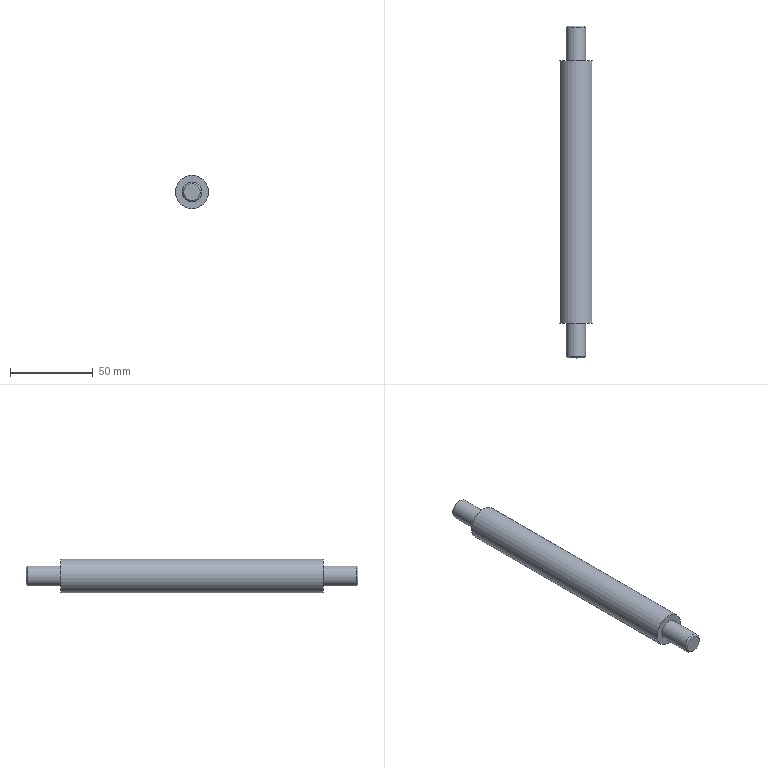Part | STEP file | YBQDJ-DX-4 | 1 solid | 9 faces | box 20 x 200 x 20 mm | volume 54352 mm3 | plane 4 | cylinder 3 | cone 2 | commonest cylinder face diameters 12 x2 20 x1
STEP:
#1=CARTESIAN_POINT('',(0.,0.,0.));
#2=DIRECTION('',(0.,0.,1.));
#3=DIRECTION('',(1.,0.,0.));
#4=AXIS2_PLACEMENT_3D('',#1,#2,#3);
#5=CARTESIAN_POINT('',(441.5,384.,130.));
#6=VERTEX_POINT('',#5);
#7=CARTESIAN_POINT('',(441.5,384.,150.));
#8=VERTEX_POINT('',#7);
#9=CARTESIAN_POINT('',(441.5,384.,140.));
#10=DIRECTION('',(0.,1.,0.));
#11=DIRECTION('',(0.,0.,1.));
#12=AXIS2_PLACEMENT_3D('',#9,#10,#11);
#13=CIRCLE('',#12,10.);
#14=CARTESIAN_POINT('',(441.5,260.,140.));
#15=DIRECTION('',(0.,1.,0.));
#16=DIRECTION('',(0.,0.,-1.));
#17=AXIS2_PLACEMENT_3D('',#14,#15,#16);
#18=CYLINDRICAL_SURFACE('',#17,10.);
#19=CARTESIAN_POINT('',(-3.142,124.));
#20=DIRECTION('',(1.,0.));
#21=VECTOR('',#20,1.);
#22=LINE('',#19,#21);
#23=(GEOMETRIC_REPRESENTATION_CONTEXT(2)PARAMETRIC_REPRESENTATION_CONTEXT()REPRESENTATION_CONTEXT('',''));
#24=DEFINITIONAL_REPRESENTATION('',(#22),#23);
#25=PCURVE('',#18,#24);
#26=CARTESIAN_POINT('',(441.5,384.,140.));
#27=DIRECTION('',(0.,1.,0.));
#28=DIRECTION('',(0.,0.,-1.));
#29=AXIS2_PLACEMENT_3D('',#26,#27,#28);
#30=PLANE('',#29);
#31=CARTESIAN_POINT('',(0.,0.));
#32=DIRECTION('',(-1.,0.));
#33=AXIS2_PLACEMENT_2D('',#31,#32);
#34=CIRCLE('',#33,10.);
#35=(GEOMETRIC_REPRESENTATION_CONTEXT(2)PARAMETRIC_REPRESENTATION_CONTEXT()REPRESENTATION_CONTEXT('',''));
#36=DEFINITIONAL_REPRESENTATION('',(#34),#35);
#37=PCURVE('',#30,#36);
#38=SURFACE_CURVE('',#13,(#25,#37),.PCURVE_S1.);
#39=EDGE_CURVE('',#6,#8,#38,.T.);
#40=ORIENTED_EDGE('',*,*,#39,.F.);
#41=CARTESIAN_POINT('',(441.5,226.,130.));
#42=VERTEX_POINT('',#41);
#43=CARTESIAN_POINT('',(441.5,226.,130.));
#44=CARTESIAN_POINT('',(441.5,384.,130.));
#45=B_SPLINE_CURVE_WITH_KNOTS('',1,(#43,#44),.UNSPECIFIED.,.F.,.F.,(2,2),(-34.,124.),.PIECEWISE_BEZIER_KNOTS.);
#46=CARTESIAN_POINT('',(0.,0.));
#47=DIRECTION('',(0.,1.));
#48=VECTOR('',#47,1.);
#49=LINE('',#46,#48);
#50=(GEOMETRIC_REPRESENTATION_CONTEXT(2)PARAMETRIC_REPRESENTATION_CONTEXT()REPRESENTATION_CONTEXT('',''));
#51=DEFINITIONAL_REPRESENTATION('',(#49),#50);
#52=PCURVE('',#18,#51);
#53=CARTESIAN_POINT('',(6.283,0.));
#54=DIRECTION('',(0.,1.));
#55=VECTOR('',#54,1.);
#56=LINE('',#53,#55);
#57=(GEOMETRIC_REPRESENTATION_CONTEXT(2)PARAMETRIC_REPRESENTATION_CONTEXT()REPRESENTATION_CONTEXT('',''));
#58=DEFINITIONAL_REPRESENTATION('',(#56),#57);
#59=PCURVE('',#18,#58);
#60=SEAM_CURVE('',#45,(#52,#59),.PCURVE_S1.);
#61=EDGE_CURVE('',#42,#6,#60,.T.);
#62=ORIENTED_EDGE('',*,*,#61,.F.);
#63=CARTESIAN_POINT('',(441.5,226.,140.));
#64=DIRECTION('',(0.,-1.,0.));
#65=DIRECTION('',(0.,0.,-1.));
#66=AXIS2_PLACEMENT_3D('',#63,#64,#65);
#67=CIRCLE('',#66,10.);
#68=CARTESIAN_POINT('',(6.283,-34.));
#69=DIRECTION('',(-1.,0.));
#70=VECTOR('',#69,1.);
#71=LINE('',#68,#70);
#72=(GEOMETRIC_REPRESENTATION_CONTEXT(2)PARAMETRIC_REPRESENTATION_CONTEXT()REPRESENTATION_CONTEXT('',''));
#73=DEFINITIONAL_REPRESENTATION('',(#71),#72);
#74=PCURVE('',#18,#73);
#75=CARTESIAN_POINT('',(441.5,226.,140.));
#76=DIRECTION('',(0.,-1.,0.));
#77=DIRECTION('',(0.,0.,-1.));
#78=AXIS2_PLACEMENT_3D('',#75,#76,#77);
#79=PLANE('',#78);
#80=CARTESIAN_POINT('',(0.,0.));
#81=DIRECTION('',(1.,0.));
#82=AXIS2_PLACEMENT_2D('',#80,#81);
#83=CIRCLE('',#82,10.);
#84=(GEOMETRIC_REPRESENTATION_CONTEXT(2)PARAMETRIC_REPRESENTATION_CONTEXT()REPRESENTATION_CONTEXT('',''));
#85=DEFINITIONAL_REPRESENTATION('',(#83),#84);
#86=PCURVE('',#79,#85);
#87=SURFACE_CURVE('',#67,(#74,#86),.PCURVE_S1.);
#88=EDGE_CURVE('',#42,#42,#87,.T.);
#89=ORIENTED_EDGE('',*,*,#88,.F.);
#90=ORIENTED_EDGE('',*,*,#61,.T.);
#91=CARTESIAN_POINT('',(441.5,384.,140.));
#92=DIRECTION('',(0.,1.,0.));
#93=DIRECTION('',(0.,0.,1.));
#94=AXIS2_PLACEMENT_3D('',#91,#92,#93);
#95=CIRCLE('',#94,10.);
#96=CARTESIAN_POINT('',(3.142,124.));
#97=DIRECTION('',(1.,0.));
#98=VECTOR('',#97,1.);
#99=LINE('',#96,#98);
#100=(GEOMETRIC_REPRESENTATION_CONTEXT(2)PARAMETRIC_REPRESENTATION_CONTEXT()REPRESENTATION_CONTEXT('',''));
#101=DEFINITIONAL_REPRESENTATION('',(#99),#100);
#102=PCURVE('',#18,#101);
#103=CARTESIAN_POINT('',(0.,0.));
#104=DIRECTION('',(-1.,0.));
#105=AXIS2_PLACEMENT_2D('',#103,#104);
#106=CIRCLE('',#105,10.);
#107=(GEOMETRIC_REPRESENTATION_CONTEXT(2)PARAMETRIC_REPRESENTATION_CONTEXT()REPRESENTATION_CONTEXT('',''));
#108=DEFINITIONAL_REPRESENTATION('',(#106),#107);
#109=PCURVE('',#30,#108);
#110=SURFACE_CURVE('',#95,(#102,#109),.PCURVE_S1.);
#111=EDGE_CURVE('',#8,#6,#110,.T.);
#112=ORIENTED_EDGE('',*,*,#111,.F.);
#113=EDGE_LOOP('',(#40,#62,#89,#90,#112));
#114=FACE_BOUND('',#113,.T.);
#115=ADVANCED_FACE('',(#114),#18,.T.);
#116=CARTESIAN_POINT('',(441.5,384.,146.));
#117=VERTEX_POINT('',#116);
#118=CARTESIAN_POINT('',(441.5,384.,140.));
#119=DIRECTION('',(0.,-1.,0.));
#120=DIRECTION('',(0.,0.,1.));
#121=AXIS2_PLACEMENT_3D('',#118,#119,#120);
#122=CIRCLE('',#121,6.);
#123=CARTESIAN_POINT('',(-6.,0.));
#124=CARTESIAN_POINT('',(-6.,10.392));
#125=CARTESIAN_POINT('',(3.,5.196));
#126=CARTESIAN_POINT('',(12.,0.));
#127=CARTESIAN_POINT('',(3.,-5.196));
#128=CARTESIAN_POINT('',(-6.,-10.392));
#129=CARTESIAN_POINT('',(-6.,0.));
#130=(BOUNDED_CURVE()B_SPLINE_CURVE(2,(#123,#124,#125,#126,#127,#128,#129),.UNSPECIFIED.,.T.,.F.)B_SPLINE_CURVE_WITH_KNOTS((1,2,2,2,2,1),(-2.094,0.,2.094,4.189,6.283,8.378),.UNSPECIFIED.)CURVE()GEOMETRIC_REPRESENTATION_ITEM()RATIONAL_B_SPLINE_CURVE((1.,0.5,1.,0.5,1.,0.5,1.))REPRESENTATION_ITEM(''));
#131=(GEOMETRIC_REPRESENTATION_CONTEXT(2)PARAMETRIC_REPRESENTATION_CONTEXT()REPRESENTATION_CONTEXT('',''));
#132=DEFINITIONAL_REPRESENTATION('',(#130),#131);
#133=PCURVE('',#30,#132);
#134=CARTESIAN_POINT('',(441.5,410.,140.));
#135=DIRECTION('',(0.,-1.,0.));
#136=DIRECTION('',(0.,0.,1.));
#137=AXIS2_PLACEMENT_3D('',#134,#135,#136);
#138=CYLINDRICAL_SURFACE('',#137,6.);
#139=CARTESIAN_POINT('',(0.,26.));
#140=DIRECTION('',(1.,0.));
#141=VECTOR('',#140,1.);
#142=LINE('',#139,#141);
#143=(GEOMETRIC_REPRESENTATION_CONTEXT(2)PARAMETRIC_REPRESENTATION_CONTEXT()REPRESENTATION_CONTEXT('',''));
#144=DEFINITIONAL_REPRESENTATION('',(#142),#143);
#145=PCURVE('',#138,#144);
#146=SURFACE_CURVE('',#122,(#133,#145),.PCURVE_S1.);
#147=EDGE_CURVE('',#117,#117,#146,.T.);
#148=ORIENTED_EDGE('',*,*,#147,.T.);
#149=EDGE_LOOP('',(#148));
#150=FACE_BOUND('',#149,.T.);
#151=ORIENTED_EDGE('',*,*,#111,.T.);
#152=ORIENTED_EDGE('',*,*,#39,.T.);
#153=EDGE_LOOP('',(#151,#152));
#154=FACE_BOUND('',#153,.T.);
#155=ADVANCED_FACE('',(#150,#154),#30,.T.);
#156=CARTESIAN_POINT('',(441.5,404.,134.));
#157=VERTEX_POINT('',#156);
#158=CARTESIAN_POINT('',(441.5,404.,146.));
#159=VERTEX_POINT('',#158);
#160=CARTESIAN_POINT('',(441.5,404.,140.));
#161=DIRECTION('',(0.,-1.,0.));
#162=DIRECTION('',(0.,0.,-1.));
#163=AXIS2_PLACEMENT_3D('',#160,#161,#162);
#164=CIRCLE('',#163,6.);
#165=CARTESIAN_POINT('',(3.142,6.));
#166=DIRECTION('',(1.,0.));
#167=VECTOR('',#166,1.);
#168=LINE('',#165,#167);
#169=(GEOMETRIC_REPRESENTATION_CONTEXT(2)PARAMETRIC_REPRESENTATION_CONTEXT()REPRESENTATION_CONTEXT('',''));
#170=DEFINITIONAL_REPRESENTATION('',(#168),#169);
#171=PCURVE('',#138,#170);
#172=CARTESIAN_POINT('',(441.5,405.,140.));
#173=DIRECTION('',(0.,-1.,0.));
#174=DIRECTION('',(0.,0.,-1.));
#175=AXIS2_PLACEMENT_3D('',#172,#173,#174);
#176=CONICAL_SURFACE('',#175,5.,0.7854);
#177=CARTESIAN_POINT('',(0.,1.));
#178=DIRECTION('',(1.,0.));
#179=VECTOR('',#178,1.);
#180=LINE('',#177,#179);
#181=(GEOMETRIC_REPRESENTATION_CONTEXT(2)PARAMETRIC_REPRESENTATION_CONTEXT()REPRESENTATION_CONTEXT('',''));
#182=DEFINITIONAL_REPRESENTATION('',(#180),#181);
#183=PCURVE('',#176,#182);
#184=SURFACE_CURVE('',#164,(#171,#183),.PCURVE_S1.);
#185=EDGE_CURVE('',#157,#159,#184,.T.);
#186=ORIENTED_EDGE('',*,*,#185,.T.);
#187=CARTESIAN_POINT('',(441.5,404.,146.));
#188=CARTESIAN_POINT('',(441.5,384.,146.));
#189=B_SPLINE_CURVE_WITH_KNOTS('',1,(#187,#188),.UNSPECIFIED.,.F.,.F.,(2,2),(6.,26.),.PIECEWISE_BEZIER_KNOTS.);
#190=CARTESIAN_POINT('',(6.283,0.));
#191=DIRECTION('',(0.,1.));
#192=VECTOR('',#191,1.);
#193=LINE('',#190,#192);
#194=(GEOMETRIC_REPRESENTATION_CONTEXT(2)PARAMETRIC_REPRESENTATION_CONTEXT()REPRESENTATION_CONTEXT('',''));
#195=DEFINITIONAL_REPRESENTATION('',(#193),#194);
#196=PCURVE('',#138,#195);
#197=CARTESIAN_POINT('',(0.,0.));
#198=DIRECTION('',(0.,1.));
#199=VECTOR('',#198,1.);
#200=LINE('',#197,#199);
#201=(GEOMETRIC_REPRESENTATION_CONTEXT(2)PARAMETRIC_REPRESENTATION_CONTEXT()REPRESENTATION_CONTEXT('',''));
#202=DEFINITIONAL_REPRESENTATION('',(#200),#201);
#203=PCURVE('',#138,#202);
#204=SEAM_CURVE('',#189,(#196,#203),.PCURVE_S1.);
#205=EDGE_CURVE('',#159,#117,#204,.T.);
#206=ORIENTED_EDGE('',*,*,#205,.T.);
#207=ORIENTED_EDGE('',*,*,#147,.F.);
#208=ORIENTED_EDGE('',*,*,#205,.F.);
#209=CARTESIAN_POINT('',(441.5,404.,140.));
#210=DIRECTION('',(0.,-1.,0.));
#211=DIRECTION('',(0.,0.,-1.));
#212=AXIS2_PLACEMENT_3D('',#209,#210,#211);
#213=CIRCLE('',#212,6.);
#214=CARTESIAN_POINT('',(-3.142,6.));
#215=DIRECTION('',(1.,0.));
#216=VECTOR('',#215,1.);
#217=LINE('',#214,#216);
#218=(GEOMETRIC_REPRESENTATION_CONTEXT(2)PARAMETRIC_REPRESENTATION_CONTEXT()REPRESENTATION_CONTEXT('',''));
#219=DEFINITIONAL_REPRESENTATION('',(#217),#218);
#220=PCURVE('',#138,#219);
#221=CARTESIAN_POINT('',(0.,1.));
#222=DIRECTION('',(1.,0.));
#223=VECTOR('',#222,1.);
#224=LINE('',#221,#223);
#225=(GEOMETRIC_REPRESENTATION_CONTEXT(2)PARAMETRIC_REPRESENTATION_CONTEXT()REPRESENTATION_CONTEXT('',''));
#226=DEFINITIONAL_REPRESENTATION('',(#224),#225);
#227=PCURVE('',#176,#226);
#228=SURFACE_CURVE('',#213,(#220,#227),.PCURVE_S1.);
#229=EDGE_CURVE('',#159,#157,#228,.T.);
#230=ORIENTED_EDGE('',*,*,#229,.T.);
#231=EDGE_LOOP('',(#186,#206,#207,#208,#230));
#232=FACE_BOUND('',#231,.T.);
#233=ADVANCED_FACE('',(#232),#138,.T.);
#234=CARTESIAN_POINT('',(446.5,405.,140.));
#235=VERTEX_POINT('',#234);
#236=CARTESIAN_POINT('',(441.5,405.,135.));
#237=VERTEX_POINT('',#236);
#238=CARTESIAN_POINT('',(441.5,405.,140.));
#239=DIRECTION('',(0.,1.,0.));
#240=DIRECTION('',(1.,0.,0.));
#241=AXIS2_PLACEMENT_3D('',#238,#239,#240);
#242=CIRCLE('',#241,5.);
#243=CARTESIAN_POINT('',(466.5,405.,20.));
#244=DIRECTION('',(0.,-1.,0.));
#245=DIRECTION('',(0.,0.,1.));
#246=AXIS2_PLACEMENT_3D('',#243,#244,#245);
#247=PLANE('',#246);
#248=CARTESIAN_POINT('',(120.,20.));
#249=CARTESIAN_POINT('',(111.34,20.));
#250=CARTESIAN_POINT('',(115.67,27.5));
#251=CARTESIAN_POINT('',(120.,35.));
#252=CARTESIAN_POINT('',(124.33,27.5));
#253=CARTESIAN_POINT('',(128.66,20.));
#254=CARTESIAN_POINT('',(120.,20.));
#255=(BOUNDED_CURVE()B_SPLINE_CURVE(2,(#248,#249,#250,#251,#252,#253,#254),.UNSPECIFIED.,.T.,.F.)B_SPLINE_CURVE_WITH_KNOTS((1,2,2,2,2,1),(-2.094,0.,2.094,4.189,6.283,8.378),.UNSPECIFIED.)CURVE()GEOMETRIC_REPRESENTATION_ITEM()RATIONAL_B_SPLINE_CURVE((1.,0.5,1.,0.5,1.,0.5,1.))REPRESENTATION_ITEM(''));
#256=(GEOMETRIC_REPRESENTATION_CONTEXT(2)PARAMETRIC_REPRESENTATION_CONTEXT()REPRESENTATION_CONTEXT('',''));
#257=DEFINITIONAL_REPRESENTATION('',(#255),#256);
#258=PCURVE('',#247,#257);
#259=CARTESIAN_POINT('',(1.571,0.));
#260=DIRECTION('',(-1.,0.));
#261=VECTOR('',#260,1.);
#262=LINE('',#259,#261);
#263=(GEOMETRIC_REPRESENTATION_CONTEXT(2)PARAMETRIC_REPRESENTATION_CONTEXT()REPRESENTATION_CONTEXT('',''));
#264=DEFINITIONAL_REPRESENTATION('',(#262),#263);
#265=PCURVE('',#176,#264);
#266=SURFACE_CURVE('',#242,(#258,#265),.PCURVE_S1.);
#267=EDGE_CURVE('',#235,#237,#266,.T.);
#268=ORIENTED_EDGE('',*,*,#267,.T.);
#269=CARTESIAN_POINT('',(441.5,405.,140.));
#270=DIRECTION('',(0.,1.,0.));
#271=DIRECTION('',(1.,0.,0.));
#272=AXIS2_PLACEMENT_3D('',#269,#270,#271);
#273=CIRCLE('',#272,5.);
#274=CARTESIAN_POINT('',(120.,20.));
#275=CARTESIAN_POINT('',(111.34,20.));
#276=CARTESIAN_POINT('',(115.67,27.5));
#277=CARTESIAN_POINT('',(120.,35.));
#278=CARTESIAN_POINT('',(124.33,27.5));
#279=CARTESIAN_POINT('',(128.66,20.));
#280=CARTESIAN_POINT('',(120.,20.));
#281=(BOUNDED_CURVE()B_SPLINE_CURVE(2,(#274,#275,#276,#277,#278,#279,#280),.UNSPECIFIED.,.T.,.F.)B_SPLINE_CURVE_WITH_KNOTS((1,2,2,2,2,1),(-2.094,0.,2.094,4.189,6.283,8.378),.UNSPECIFIED.)CURVE()GEOMETRIC_REPRESENTATION_ITEM()RATIONAL_B_SPLINE_CURVE((1.,0.5,1.,0.5,1.,0.5,1.))REPRESENTATION_ITEM(''));
#282=(GEOMETRIC_REPRESENTATION_CONTEXT(2)PARAMETRIC_REPRESENTATION_CONTEXT()REPRESENTATION_CONTEXT('',''));
#283=DEFINITIONAL_REPRESENTATION('',(#281),#282);
#284=PCURVE('',#247,#283);
#285=CARTESIAN_POINT('',(7.854,0.));
#286=DIRECTION('',(-1.,0.));
#287=VECTOR('',#286,1.);
#288=LINE('',#285,#287);
#289=(GEOMETRIC_REPRESENTATION_CONTEXT(2)PARAMETRIC_REPRESENTATION_CONTEXT()REPRESENTATION_CONTEXT('',''));
#290=DEFINITIONAL_REPRESENTATION('',(#288),#289);
#291=PCURVE('',#176,#290);
#292=SURFACE_CURVE('',#273,(#284,#291),.PCURVE_S1.);
#293=EDGE_CURVE('',#237,#235,#292,.T.);
#294=ORIENTED_EDGE('',*,*,#293,.T.);
#295=EDGE_LOOP('',(#268,#294));
#296=FACE_BOUND('',#295,.T.);
#297=ADVANCED_FACE('',(#296),#247,.F.);
#298=CARTESIAN_POINT('',(441.5,226.,134.));
#299=VERTEX_POINT('',#298);
#300=CARTESIAN_POINT('',(441.5,226.,146.));
#301=VERTEX_POINT('',#300);
#302=CARTESIAN_POINT('',(441.5,226.,140.));
#303=DIRECTION('',(0.,1.,0.));
#304=DIRECTION('',(0.,0.,-1.));
#305=AXIS2_PLACEMENT_3D('',#302,#303,#304);
#306=CIRCLE('',#305,6.);
#307=CARTESIAN_POINT('',(6.,0.));
#308=CARTESIAN_POINT('',(6.,-10.392));
#309=CARTESIAN_POINT('',(-3.,-5.196));
#310=CARTESIAN_POINT('',(-12.,0.));
#311=CARTESIAN_POINT('',(-3.,5.196));
#312=CARTESIAN_POINT('',(6.,10.392));
#313=CARTESIAN_POINT('',(6.,0.));
#314=(BOUNDED_CURVE()B_SPLINE_CURVE(2,(#307,#308,#309,#310,#311,#312,#313),.UNSPECIFIED.,.T.,.F.)B_SPLINE_CURVE_WITH_KNOTS((1,2,2,2,2,1),(-2.094,0.,2.094,4.189,6.283,8.378),.UNSPECIFIED.)CURVE()GEOMETRIC_REPRESENTATION_ITEM()RATIONAL_B_SPLINE_CURVE((1.,0.5,1.,0.5,1.,0.5,1.))REPRESENTATION_ITEM(''));
#315=(GEOMETRIC_REPRESENTATION_CONTEXT(2)PARAMETRIC_REPRESENTATION_CONTEXT()REPRESENTATION_CONTEXT('',''));
#316=DEFINITIONAL_REPRESENTATION('',(#314),#315);
#317=PCURVE('',#79,#316);
#318=CARTESIAN_POINT('',(441.5,200.,140.));
#319=DIRECTION('',(0.,1.,0.));
#320=DIRECTION('',(0.,0.,1.));
#321=AXIS2_PLACEMENT_3D('',#318,#319,#320);
#322=CYLINDRICAL_SURFACE('',#321,6.);
#323=CARTESIAN_POINT('',(3.142,26.));
#324=DIRECTION('',(1.,0.));
#325=VECTOR('',#324,1.);
#326=LINE('',#323,#325);
#327=(GEOMETRIC_REPRESENTATION_CONTEXT(2)PARAMETRIC_REPRESENTATION_CONTEXT()REPRESENTATION_CONTEXT('',''));
#328=DEFINITIONAL_REPRESENTATION('',(#326),#327);
#329=PCURVE('',#322,#328);
#330=SURFACE_CURVE('',#306,(#317,#329),.PCURVE_S1.);
#331=EDGE_CURVE('',#299,#301,#330,.T.);
#332=ORIENTED_EDGE('',*,*,#331,.T.);
#333=CARTESIAN_POINT('',(441.5,226.,140.));
#334=DIRECTION('',(0.,1.,0.));
#335=DIRECTION('',(0.,0.,-1.));
#336=AXIS2_PLACEMENT_3D('',#333,#334,#335);
#337=CIRCLE('',#336,6.);
#338=CARTESIAN_POINT('',(6.,0.));
#339=CARTESIAN_POINT('',(6.,-10.392));
#340=CARTESIAN_POINT('',(-3.,-5.196));
#341=CARTESIAN_POINT('',(-12.,0.));
#342=CARTESIAN_POINT('',(-3.,5.196));
#343=CARTESIAN_POINT('',(6.,10.392));
#344=CARTESIAN_POINT('',(6.,0.));
#345=(BOUNDED_CURVE()B_SPLINE_CURVE(2,(#338,#339,#340,#341,#342,#343,#344),.UNSPECIFIED.,.T.,.F.)B_SPLINE_CURVE_WITH_KNOTS((1,2,2,2,2,1),(-2.094,0.,2.094,4.189,6.283,8.378),.UNSPECIFIED.)CURVE()GEOMETRIC_REPRESENTATION_ITEM()RATIONAL_B_SPLINE_CURVE((1.,0.5,1.,0.5,1.,0.5,1.))REPRESENTATION_ITEM(''));
#346=(GEOMETRIC_REPRESENTATION_CONTEXT(2)PARAMETRIC_REPRESENTATION_CONTEXT()REPRESENTATION_CONTEXT('',''));
#347=DEFINITIONAL_REPRESENTATION('',(#345),#346);
#348=PCURVE('',#79,#347);
#349=CARTESIAN_POINT('',(-3.142,26.));
#350=DIRECTION('',(1.,0.));
#351=VECTOR('',#350,1.);
#352=LINE('',#349,#351);
#353=(GEOMETRIC_REPRESENTATION_CONTEXT(2)PARAMETRIC_REPRESENTATION_CONTEXT()REPRESENTATION_CONTEXT('',''));
#354=DEFINITIONAL_REPRESENTATION('',(#352),#353);
#355=PCURVE('',#322,#354);
#356=SURFACE_CURVE('',#337,(#348,#355),.PCURVE_S1.);
#357=EDGE_CURVE('',#301,#299,#356,.T.);
#358=ORIENTED_EDGE('',*,*,#357,.T.);
#359=EDGE_LOOP('',(#332,#358));
#360=FACE_BOUND('',#359,.T.);
#361=ORIENTED_EDGE('',*,*,#88,.T.);
#362=EDGE_LOOP('',(#361));
#363=FACE_BOUND('',#362,.T.);
#364=ADVANCED_FACE('',(#360,#363),#79,.T.);
#365=CARTESIAN_POINT('',(441.5,206.,146.));
#366=VERTEX_POINT('',#365);
#367=CARTESIAN_POINT('',(441.5,206.,140.));
#368=DIRECTION('',(0.,1.,0.));
#369=DIRECTION('',(0.,0.,1.));
#370=AXIS2_PLACEMENT_3D('',#367,#368,#369);
#371=CIRCLE('',#370,6.);
#372=CARTESIAN_POINT('',(0.,6.));
#373=DIRECTION('',(1.,0.));
#374=VECTOR('',#373,1.);
#375=LINE('',#372,#374);
#376=(GEOMETRIC_REPRESENTATION_CONTEXT(2)PARAMETRIC_REPRESENTATION_CONTEXT()REPRESENTATION_CONTEXT('',''));
#377=DEFINITIONAL_REPRESENTATION('',(#375),#376);
#378=PCURVE('',#322,#377);
#379=CARTESIAN_POINT('',(441.5,205.,140.));
#380=DIRECTION('',(0.,1.,0.));
#381=DIRECTION('',(0.,0.,1.));
#382=AXIS2_PLACEMENT_3D('',#379,#380,#381);
#383=CONICAL_SURFACE('',#382,5.,0.7854);
#384=CARTESIAN_POINT('',(0.,1.));
#385=DIRECTION('',(1.,0.));
#386=VECTOR('',#385,1.);
#387=LINE('',#384,#386);
#388=(GEOMETRIC_REPRESENTATION_CONTEXT(2)PARAMETRIC_REPRESENTATION_CONTEXT()REPRESENTATION_CONTEXT('',''));
#389=DEFINITIONAL_REPRESENTATION('',(#387),#388);
#390=PCURVE('',#383,#389);
#391=SURFACE_CURVE('',#371,(#378,#390),.PCURVE_S1.);
#392=EDGE_CURVE('',#366,#366,#391,.T.);
#393=ORIENTED_EDGE('',*,*,#392,.T.);
#394=CARTESIAN_POINT('',(441.5,206.,146.));
#395=CARTESIAN_POINT('',(441.5,226.,146.));
#396=B_SPLINE_CURVE_WITH_KNOTS('',1,(#394,#395),.UNSPECIFIED.,.F.,.F.,(2,2),(6.,26.),.PIECEWISE_BEZIER_KNOTS.);
#397=CARTESIAN_POINT('',(6.283,0.));
#398=DIRECTION('',(0.,1.));
#399=VECTOR('',#398,1.);
#400=LINE('',#397,#399);
#401=(GEOMETRIC_REPRESENTATION_CONTEXT(2)PARAMETRIC_REPRESENTATION_CONTEXT()REPRESENTATION_CONTEXT('',''));
#402=DEFINITIONAL_REPRESENTATION('',(#400),#401);
#403=PCURVE('',#322,#402);
#404=CARTESIAN_POINT('',(0.,0.));
#405=DIRECTION('',(0.,1.));
#406=VECTOR('',#405,1.);
#407=LINE('',#404,#406);
#408=(GEOMETRIC_REPRESENTATION_CONTEXT(2)PARAMETRIC_REPRESENTATION_CONTEXT()REPRESENTATION_CONTEXT('',''));
#409=DEFINITIONAL_REPRESENTATION('',(#407),#408);
#410=PCURVE('',#322,#409);
#411=SEAM_CURVE('',#396,(#403,#410),.PCURVE_S1.);
#412=EDGE_CURVE('',#366,#301,#411,.T.);
#413=ORIENTED_EDGE('',*,*,#412,.T.);
#414=ORIENTED_EDGE('',*,*,#331,.F.);
#415=ORIENTED_EDGE('',*,*,#357,.F.);
#416=ORIENTED_EDGE('',*,*,#412,.F.);
#417=EDGE_LOOP('',(#393,#413,#414,#415,#416));
#418=FACE_BOUND('',#417,.T.);
#419=ADVANCED_FACE('',(#418),#322,.T.);
#420=CARTESIAN_POINT('',(441.5,205.,145.));
#421=VERTEX_POINT('',#420);
#422=CARTESIAN_POINT('',(441.5,205.,140.));
#423=DIRECTION('',(0.,-1.,0.));
#424=DIRECTION('',(0.,0.,1.));
#425=AXIS2_PLACEMENT_3D('',#422,#423,#424);
#426=CIRCLE('',#425,5.);
#427=CARTESIAN_POINT('',(466.5,205.,20.));
#428=DIRECTION('',(0.,1.,0.));
#429=DIRECTION('',(0.,0.,1.));
#430=AXIS2_PLACEMENT_3D('',#427,#428,#429);
#431=PLANE('',#430);
#432=CARTESIAN_POINT('',(125.,-25.));
#433=CARTESIAN_POINT('',(125.,-33.66));
#434=CARTESIAN_POINT('',(117.5,-29.33));
#435=CARTESIAN_POINT('',(110.,-25.));
#436=CARTESIAN_POINT('',(117.5,-20.67));
#437=CARTESIAN_POINT('',(125.,-16.34));
#438=CARTESIAN_POINT('',(125.,-25.));
#439=(BOUNDED_CURVE()B_SPLINE_CURVE(2,(#432,#433,#434,#435,#436,#437,#438),.UNSPECIFIED.,.T.,.F.)B_SPLINE_CURVE_WITH_KNOTS((1,2,2,2,2,1),(-2.094,0.,2.094,4.189,6.283,8.378),.UNSPECIFIED.)CURVE()GEOMETRIC_REPRESENTATION_ITEM()RATIONAL_B_SPLINE_CURVE((1.,0.5,1.,0.5,1.,0.5,1.))REPRESENTATION_ITEM(''));
#440=(GEOMETRIC_REPRESENTATION_CONTEXT(2)PARAMETRIC_REPRESENTATION_CONTEXT()REPRESENTATION_CONTEXT('',''));
#441=DEFINITIONAL_REPRESENTATION('',(#439),#440);
#442=PCURVE('',#431,#441);
#443=CARTESIAN_POINT('',(6.283,0.));
#444=DIRECTION('',(-1.,0.));
#445=VECTOR('',#444,1.);
#446=LINE('',#443,#445);
#447=(GEOMETRIC_REPRESENTATION_CONTEXT(2)PARAMETRIC_REPRESENTATION_CONTEXT()REPRESENTATION_CONTEXT('',''));
#448=DEFINITIONAL_REPRESENTATION('',(#446),#447);
#449=PCURVE('',#383,#448);
#450=SURFACE_CURVE('',#426,(#442,#449),.PCURVE_S1.);
#451=EDGE_CURVE('',#421,#421,#450,.T.);
#452=ORIENTED_EDGE('',*,*,#451,.T.);
#453=EDGE_LOOP('',(#452));
#454=FACE_BOUND('',#453,.T.);
#455=ADVANCED_FACE('',(#454),#431,.F.);
#456=ORIENTED_EDGE('',*,*,#392,.F.);
#457=CARTESIAN_POINT('',(441.5,205.,145.));
#458=CARTESIAN_POINT('',(441.5,206.,146.));
#459=B_SPLINE_CURVE_WITH_KNOTS('',1,(#457,#458),.UNSPECIFIED.,.F.,.F.,(2,2),(0.,1.414),.PIECEWISE_BEZIER_KNOTS.);
#460=CARTESIAN_POINT('',(0.,0.));
#461=DIRECTION('',(0.,1.));
#462=VECTOR('',#461,1.);
#463=LINE('',#460,#462);
#464=(GEOMETRIC_REPRESENTATION_CONTEXT(2)PARAMETRIC_REPRESENTATION_CONTEXT()REPRESENTATION_CONTEXT('',''));
#465=DEFINITIONAL_REPRESENTATION('',(#463),#464);
#466=PCURVE('',#383,#465);
#467=CARTESIAN_POINT('',(6.283,0.));
#468=DIRECTION('',(0.,1.));
#469=VECTOR('',#468,1.);
#470=LINE('',#467,#469);
#471=(GEOMETRIC_REPRESENTATION_CONTEXT(2)PARAMETRIC_REPRESENTATION_CONTEXT()REPRESENTATION_CONTEXT('',''));
#472=DEFINITIONAL_REPRESENTATION('',(#470),#471);
#473=PCURVE('',#383,#472);
#474=SEAM_CURVE('',#459,(#466,#473),.PCURVE_S1.);
#475=EDGE_CURVE('',#421,#366,#474,.T.);
#476=ORIENTED_EDGE('',*,*,#475,.F.);
#477=ORIENTED_EDGE('',*,*,#451,.F.);
#478=ORIENTED_EDGE('',*,*,#475,.T.);
#479=EDGE_LOOP('',(#456,#476,#477,#478));
#480=FACE_BOUND('',#479,.T.);
#481=ADVANCED_FACE('',(#480),#383,.T.);
#482=ORIENTED_EDGE('',*,*,#185,.F.);
#483=CARTESIAN_POINT('',(441.5,405.,135.));
#484=CARTESIAN_POINT('',(441.5,404.,134.));
#485=B_SPLINE_CURVE_WITH_KNOTS('',1,(#483,#484),.UNSPECIFIED.,.F.,.F.,(2,2),(0.,1.414),.PIECEWISE_BEZIER_KNOTS.);
#486=CARTESIAN_POINT('',(0.,0.));
#487=DIRECTION('',(0.,1.));
#488=VECTOR('',#487,1.);
#489=LINE('',#486,#488);
#490=(GEOMETRIC_REPRESENTATION_CONTEXT(2)PARAMETRIC_REPRESENTATION_CONTEXT()REPRESENTATION_CONTEXT('',''));
#491=DEFINITIONAL_REPRESENTATION('',(#489),#490);
#492=PCURVE('',#176,#491);
#493=CARTESIAN_POINT('',(6.283,0.));
#494=DIRECTION('',(0.,1.));
#495=VECTOR('',#494,1.);
#496=LINE('',#493,#495);
#497=(GEOMETRIC_REPRESENTATION_CONTEXT(2)PARAMETRIC_REPRESENTATION_CONTEXT()REPRESENTATION_CONTEXT('',''));
#498=DEFINITIONAL_REPRESENTATION('',(#496),#497);
#499=PCURVE('',#176,#498);
#500=SEAM_CURVE('',#485,(#492,#499),.PCURVE_S1.);
#501=EDGE_CURVE('',#237,#157,#500,.T.);
#502=ORIENTED_EDGE('',*,*,#501,.F.);
#503=ORIENTED_EDGE('',*,*,#267,.F.);
#504=ORIENTED_EDGE('',*,*,#293,.F.);
#505=ORIENTED_EDGE('',*,*,#501,.T.);
#506=ORIENTED_EDGE('',*,*,#229,.F.);
#507=EDGE_LOOP('',(#482,#502,#503,#504,#505,#506));
#508=FACE_BOUND('',#507,.T.);
#509=ADVANCED_FACE('',(#508),#176,.T.);
#510=CLOSED_SHELL('',(#115,#155,#233,#297,#364,#419,#455,#481,#509));
#511=MANIFOLD_SOLID_BREP('',#510);
#512=(LENGTH_UNIT()NAMED_UNIT(*)SI_UNIT(.MILLI.,.METRE.));
#513=UNCERTAINTY_MEASURE_WITH_UNIT(LENGTH_MEASURE(0.000005),#512,'','');
#514=(NAMED_UNIT(*)PLANE_ANGLE_UNIT()SI_UNIT($,.RADIAN.));
#515=(NAMED_UNIT(*)SI_UNIT($,.STERADIAN.)SOLID_ANGLE_UNIT());
#516=(GEOMETRIC_REPRESENTATION_CONTEXT(3)GLOBAL_UNCERTAINTY_ASSIGNED_CONTEXT((#513))GLOBAL_UNIT_ASSIGNED_CONTEXT((#512,#514,#515))REPRESENTATION_CONTEXT('',''));
#517=ADVANCED_BREP_SHAPE_REPRESENTATION('',(#4,#511),#516);